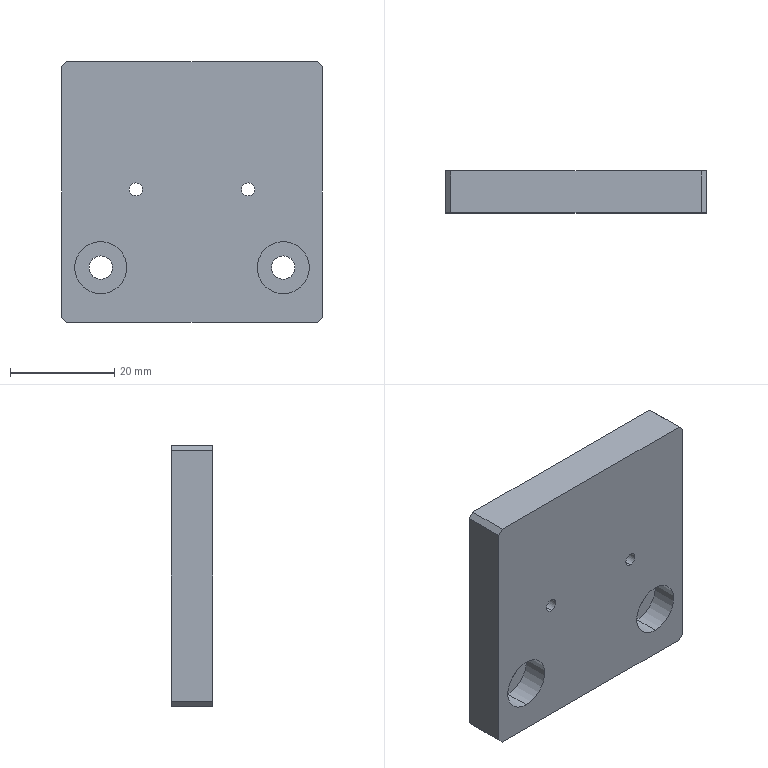Part | NX | features BREP 1 | 1 solid | 24 faces | box 50 x 8 x 50 mm | volume 19025 mm3 | plane 12 | cylinder 12 | commonest cylinder face diameters 2.5 x4 4.5 x4 10 x4
STEP:
#1=CARTESIAN_POINT('',(24.,8.,25.));
#2=VERTEX_POINT('',#1);
#3=CARTESIAN_POINT('',(25.,8.,24.));
#4=VERTEX_POINT('',#3);
#5=CARTESIAN_POINT('',(24.5,8.,24.5));
#6=DIRECTION('',(0.7071,0.,-0.7071));
#7=VECTOR('',#6,1000.);
#8=LINE('',#5,#7);
#9=EDGE_CURVE('',#2,#4,#8,.T.);
#10=ORIENTED_EDGE('',*,*,#9,.F.);
#11=CARTESIAN_POINT('',(24.,0.,25.));
#12=VERTEX_POINT('',#11);
#13=CARTESIAN_POINT('',(24.,8.,25.));
#14=DIRECTION('',(0.,1.,0.));
#15=VECTOR('',#14,1000.);
#16=LINE('',#13,#15);
#17=EDGE_CURVE('',#12,#2,#16,.T.);
#18=ORIENTED_EDGE('',*,*,#17,.F.);
#19=CARTESIAN_POINT('',(25.,0.,24.));
#20=VERTEX_POINT('',#19);
#21=CARTESIAN_POINT('',(25.,0.,24.));
#22=DIRECTION('',(-0.7071,0.,0.7071));
#23=VECTOR('',#22,1000.);
#24=LINE('',#21,#23);
#25=EDGE_CURVE('',#20,#12,#24,.T.);
#26=ORIENTED_EDGE('',*,*,#25,.F.);
#27=CARTESIAN_POINT('',(25.,8.,24.));
#28=DIRECTION('',(0.,-1.,0.));
#29=VECTOR('',#28,1000.);
#30=LINE('',#27,#29);
#31=EDGE_CURVE('',#4,#20,#30,.T.);
#32=ORIENTED_EDGE('',*,*,#31,.F.);
#33=EDGE_LOOP('',(#10,#18,#26,#32));
#34=FACE_BOUND('',#33,.T.);
#35=CARTESIAN_POINT('',(25.,8.,24.));
#36=DIRECTION('',(-0.7071,0.,-0.7071));
#37=DIRECTION('',(0.,-1.,0.));
#38=AXIS2_PLACEMENT_3D('',#35,#36,#37);
#39=PLANE('',#38);
#40=ADVANCED_FACE('',(#34),#39,.F.);
#41=CARTESIAN_POINT('',(-25.,8.,24.));
#42=VERTEX_POINT('',#41);
#43=CARTESIAN_POINT('',(-24.,8.,25.));
#44=VERTEX_POINT('',#43);
#45=CARTESIAN_POINT('',(-24.5,8.,24.5));
#46=DIRECTION('',(0.7071,0.,0.7071));
#47=VECTOR('',#46,1000.);
#48=LINE('',#45,#47);
#49=EDGE_CURVE('',#42,#44,#48,.T.);
#50=ORIENTED_EDGE('',*,*,#49,.F.);
#51=CARTESIAN_POINT('',(-25.,0.,24.));
#52=VERTEX_POINT('',#51);
#53=CARTESIAN_POINT('',(-25.,8.,24.));
#54=DIRECTION('',(0.,1.,0.));
#55=VECTOR('',#54,1000.);
#56=LINE('',#53,#55);
#57=EDGE_CURVE('',#52,#42,#56,.T.);
#58=ORIENTED_EDGE('',*,*,#57,.F.);
#59=CARTESIAN_POINT('',(-24.,0.,25.));
#60=VERTEX_POINT('',#59);
#61=CARTESIAN_POINT('',(-24.,0.,25.));
#62=DIRECTION('',(-0.7071,0.,-0.7071));
#63=VECTOR('',#62,1000.);
#64=LINE('',#61,#63);
#65=EDGE_CURVE('',#60,#52,#64,.T.);
#66=ORIENTED_EDGE('',*,*,#65,.F.);
#67=CARTESIAN_POINT('',(-24.,8.,25.));
#68=DIRECTION('',(0.,-1.,0.));
#69=VECTOR('',#68,1000.);
#70=LINE('',#67,#69);
#71=EDGE_CURVE('',#44,#60,#70,.T.);
#72=ORIENTED_EDGE('',*,*,#71,.F.);
#73=EDGE_LOOP('',(#50,#58,#66,#72));
#74=FACE_BOUND('',#73,.T.);
#75=CARTESIAN_POINT('',(-24.,8.,25.));
#76=DIRECTION('',(0.7071,0.,-0.7071));
#77=DIRECTION('',(0.,-1.,0.));
#78=AXIS2_PLACEMENT_3D('',#75,#76,#77);
#79=PLANE('',#78);
#80=ADVANCED_FACE('',(#74),#79,.F.);
#81=CARTESIAN_POINT('',(-24.,8.,-25.));
#82=VERTEX_POINT('',#81);
#83=CARTESIAN_POINT('',(-25.,8.,-24.));
#84=VERTEX_POINT('',#83);
#85=CARTESIAN_POINT('',(-24.5,8.,-24.5));
#86=DIRECTION('',(-0.7071,0.,0.7071));
#87=VECTOR('',#86,1000.);
#88=LINE('',#85,#87);
#89=EDGE_CURVE('',#82,#84,#88,.T.);
#90=ORIENTED_EDGE('',*,*,#89,.F.);
#91=CARTESIAN_POINT('',(-24.,0.,-25.));
#92=VERTEX_POINT('',#91);
#93=CARTESIAN_POINT('',(-24.,8.,-25.));
#94=DIRECTION('',(0.,1.,0.));
#95=VECTOR('',#94,1000.);
#96=LINE('',#93,#95);
#97=EDGE_CURVE('',#92,#82,#96,.T.);
#98=ORIENTED_EDGE('',*,*,#97,.F.);
#99=CARTESIAN_POINT('',(-25.,0.,-24.));
#100=VERTEX_POINT('',#99);
#101=CARTESIAN_POINT('',(-25.,0.,-24.));
#102=DIRECTION('',(0.7071,0.,-0.7071));
#103=VECTOR('',#102,1000.);
#104=LINE('',#101,#103);
#105=EDGE_CURVE('',#100,#92,#104,.T.);
#106=ORIENTED_EDGE('',*,*,#105,.F.);
#107=CARTESIAN_POINT('',(-25.,8.,-24.));
#108=DIRECTION('',(0.,-1.,0.));
#109=VECTOR('',#108,1000.);
#110=LINE('',#107,#109);
#111=EDGE_CURVE('',#84,#100,#110,.T.);
#112=ORIENTED_EDGE('',*,*,#111,.F.);
#113=EDGE_LOOP('',(#90,#98,#106,#112));
#114=FACE_BOUND('',#113,.T.);
#115=CARTESIAN_POINT('',(-25.,8.,-24.));
#116=DIRECTION('',(0.7071,0.,0.7071));
#117=DIRECTION('',(0.,-1.,0.));
#118=AXIS2_PLACEMENT_3D('',#115,#116,#117);
#119=PLANE('',#118);
#120=ADVANCED_FACE('',(#114),#119,.F.);
#121=CARTESIAN_POINT('',(25.,8.,-24.));
#122=VERTEX_POINT('',#121);
#123=CARTESIAN_POINT('',(24.,8.,-25.));
#124=VERTEX_POINT('',#123);
#125=CARTESIAN_POINT('',(24.5,8.,-24.5));
#126=DIRECTION('',(-0.7071,0.,-0.7071));
#127=VECTOR('',#126,1000.);
#128=LINE('',#125,#127);
#129=EDGE_CURVE('',#122,#124,#128,.T.);
#130=ORIENTED_EDGE('',*,*,#129,.F.);
#131=CARTESIAN_POINT('',(25.,0.,-24.));
#132=VERTEX_POINT('',#131);
#133=CARTESIAN_POINT('',(25.,8.,-24.));
#134=DIRECTION('',(0.,1.,0.));
#135=VECTOR('',#134,1000.);
#136=LINE('',#133,#135);
#137=EDGE_CURVE('',#132,#122,#136,.T.);
#138=ORIENTED_EDGE('',*,*,#137,.F.);
#139=CARTESIAN_POINT('',(24.,0.,-25.));
#140=VERTEX_POINT('',#139);
#141=CARTESIAN_POINT('',(24.,0.,-25.));
#142=DIRECTION('',(0.7071,0.,0.7071));
#143=VECTOR('',#142,1000.);
#144=LINE('',#141,#143);
#145=EDGE_CURVE('',#140,#132,#144,.T.);
#146=ORIENTED_EDGE('',*,*,#145,.F.);
#147=CARTESIAN_POINT('',(24.,8.,-25.));
#148=DIRECTION('',(0.,-1.,0.));
#149=VECTOR('',#148,1000.);
#150=LINE('',#147,#149);
#151=EDGE_CURVE('',#124,#140,#150,.T.);
#152=ORIENTED_EDGE('',*,*,#151,.F.);
#153=EDGE_LOOP('',(#130,#138,#146,#152));
#154=FACE_BOUND('',#153,.T.);
#155=CARTESIAN_POINT('',(24.,8.,-25.));
#156=DIRECTION('',(-0.7071,0.,0.7071));
#157=DIRECTION('',(0.,-1.,0.));
#158=AXIS2_PLACEMENT_3D('',#155,#156,#157);
#159=PLANE('',#158);
#160=ADVANCED_FACE('',(#154),#159,.F.);
#161=CARTESIAN_POINT('',(10.75,8.,1.75));
#162=VERTEX_POINT('',#161);
#163=CARTESIAN_POINT('',(10.75,0.,1.75));
#164=VERTEX_POINT('',#163);
#165=CARTESIAN_POINT('',(10.75,0.,1.75));
#166=DIRECTION('',(0.,-1.,0.));
#167=VECTOR('',#166,1000.);
#168=LINE('',#165,#167);
#169=EDGE_CURVE('',#162,#164,#168,.T.);
#170=ORIENTED_EDGE('',*,*,#169,.F.);
#171=CARTESIAN_POINT('',(10.75,8.,-0.75));
#172=VERTEX_POINT('',#171);
#173=CARTESIAN_POINT('',(10.75,8.,0.5));
#174=DIRECTION('',(0.,-1.,0.));
#175=DIRECTION('',(0.,0.,-1.));
#176=AXIS2_PLACEMENT_3D('',#173,#174,#175);
#177=CIRCLE('',#176,1.25);
#178=EDGE_CURVE('',#172,#162,#177,.T.);
#179=ORIENTED_EDGE('',*,*,#178,.F.);
#180=CARTESIAN_POINT('',(10.75,0.,-0.75));
#181=VERTEX_POINT('',#180);
#182=CARTESIAN_POINT('',(10.75,0.,-0.75));
#183=DIRECTION('',(0.,-1.,0.));
#184=VECTOR('',#183,1000.);
#185=LINE('',#182,#184);
#186=EDGE_CURVE('',#172,#181,#185,.T.);
#187=ORIENTED_EDGE('',*,*,#186,.T.);
#188=CARTESIAN_POINT('',(10.75,0.,0.5));
#189=DIRECTION('',(0.,-1.,0.));
#190=DIRECTION('',(0.,0.,-1.));
#191=AXIS2_PLACEMENT_3D('',#188,#189,#190);
#192=CIRCLE('',#191,1.25);
#193=EDGE_CURVE('',#181,#164,#192,.T.);
#194=ORIENTED_EDGE('',*,*,#193,.T.);
#195=EDGE_LOOP('',(#170,#179,#187,#194));
#196=FACE_BOUND('',#195,.T.);
#197=CARTESIAN_POINT('',(10.75,0.,0.5));
#198=DIRECTION('',(0.,-1.,0.));
#199=DIRECTION('',(0.,0.,-1.));
#200=AXIS2_PLACEMENT_3D('',#197,#198,#199);
#201=CYLINDRICAL_SURFACE('',#200,1.25);
#202=ADVANCED_FACE('',(#196),#201,.F.);
#203=CARTESIAN_POINT('',(-10.75,8.,1.75));
#204=VERTEX_POINT('',#203);
#205=CARTESIAN_POINT('',(-10.75,0.,1.75));
#206=VERTEX_POINT('',#205);
#207=CARTESIAN_POINT('',(-10.75,0.,1.75));
#208=DIRECTION('',(0.,-1.,0.));
#209=VECTOR('',#208,1000.);
#210=LINE('',#207,#209);
#211=EDGE_CURVE('',#204,#206,#210,.T.);
#212=ORIENTED_EDGE('',*,*,#211,.F.);
#213=CARTESIAN_POINT('',(-10.75,8.,-0.75));
#214=VERTEX_POINT('',#213);
#215=CARTESIAN_POINT('',(-10.75,8.,0.5));
#216=DIRECTION('',(0.,-1.,0.));
#217=DIRECTION('',(0.,0.,-1.));
#218=AXIS2_PLACEMENT_3D('',#215,#216,#217);
#219=CIRCLE('',#218,1.25);
#220=EDGE_CURVE('',#214,#204,#219,.T.);
#221=ORIENTED_EDGE('',*,*,#220,.F.);
#222=CARTESIAN_POINT('',(-10.75,0.,-0.75));
#223=VERTEX_POINT('',#222);
#224=CARTESIAN_POINT('',(-10.75,0.,-0.75));
#225=DIRECTION('',(0.,-1.,0.));
#226=VECTOR('',#225,1000.);
#227=LINE('',#224,#226);
#228=EDGE_CURVE('',#214,#223,#227,.T.);
#229=ORIENTED_EDGE('',*,*,#228,.T.);
#230=CARTESIAN_POINT('',(-10.75,0.,0.5));
#231=DIRECTION('',(0.,-1.,0.));
#232=DIRECTION('',(0.,0.,-1.));
#233=AXIS2_PLACEMENT_3D('',#230,#231,#232);
#234=CIRCLE('',#233,1.25);
#235=EDGE_CURVE('',#223,#206,#234,.T.);
#236=ORIENTED_EDGE('',*,*,#235,.T.);
#237=EDGE_LOOP('',(#212,#221,#229,#236));
#238=FACE_BOUND('',#237,.T.);
#239=CARTESIAN_POINT('',(-10.75,0.,0.5));
#240=DIRECTION('',(0.,-1.,0.));
#241=DIRECTION('',(0.,0.,-1.));
#242=AXIS2_PLACEMENT_3D('',#239,#240,#241);
#243=CYLINDRICAL_SURFACE('',#242,1.25);
#244=ADVANCED_FACE('',(#238),#243,.F.);
#245=CARTESIAN_POINT('',(17.5,5.,-9.5));
#246=VERTEX_POINT('',#245);
#247=CARTESIAN_POINT('',(17.5,0.,-9.5));
#248=VERTEX_POINT('',#247);
#249=CARTESIAN_POINT('',(17.5,0.,-9.5));
#250=DIRECTION('',(0.,-1.,0.));
#251=VECTOR('',#250,1000.);
#252=LINE('',#249,#251);
#253=EDGE_CURVE('',#246,#248,#252,.T.);
#254=ORIENTED_EDGE('',*,*,#253,.F.);
#255=CARTESIAN_POINT('',(17.5,5.,-19.5));
#256=VERTEX_POINT('',#255);
#257=CARTESIAN_POINT('',(17.5,5.,-14.5));
#258=DIRECTION('',(0.,-1.,0.));
#259=DIRECTION('',(0.,0.,-1.));
#260=AXIS2_PLACEMENT_3D('',#257,#258,#259);
#261=CIRCLE('',#260,5.);
#262=EDGE_CURVE('',#256,#246,#261,.T.);
#263=ORIENTED_EDGE('',*,*,#262,.F.);
#264=CARTESIAN_POINT('',(17.5,0.,-19.5));
#265=VERTEX_POINT('',#264);
#266=CARTESIAN_POINT('',(17.5,0.,-19.5));
#267=DIRECTION('',(0.,-1.,0.));
#268=VECTOR('',#267,1000.);
#269=LINE('',#266,#268);
#270=EDGE_CURVE('',#256,#265,#269,.T.);
#271=ORIENTED_EDGE('',*,*,#270,.T.);
#272=CARTESIAN_POINT('',(17.5,0.,-14.5));
#273=DIRECTION('',(0.,-1.,0.));
#274=DIRECTION('',(0.,0.,-1.));
#275=AXIS2_PLACEMENT_3D('',#272,#273,#274);
#276=CIRCLE('',#275,5.);
#277=EDGE_CURVE('',#265,#248,#276,.T.);
#278=ORIENTED_EDGE('',*,*,#277,.T.);
#279=EDGE_LOOP('',(#254,#263,#271,#278));
#280=FACE_BOUND('',#279,.T.);
#281=CARTESIAN_POINT('',(17.5,0.,-14.5));
#282=DIRECTION('',(0.,-1.,0.));
#283=DIRECTION('',(0.,0.,-1.));
#284=AXIS2_PLACEMENT_3D('',#281,#282,#283);
#285=CYLINDRICAL_SURFACE('',#284,5.);
#286=ADVANCED_FACE('',(#280),#285,.F.);
#287=ORIENTED_EDGE('',*,*,#262,.T.);
#288=CARTESIAN_POINT('',(17.5,5.,-14.5));
#289=DIRECTION('',(0.,-1.,0.));
#290=DIRECTION('',(0.,0.,-1.));
#291=AXIS2_PLACEMENT_3D('',#288,#289,#290);
#292=CIRCLE('',#291,5.);
#293=EDGE_CURVE('',#246,#256,#292,.T.);
#294=ORIENTED_EDGE('',*,*,#293,.T.);
#295=EDGE_LOOP('',(#287,#294));
#296=FACE_BOUND('',#295,.T.);
#297=CARTESIAN_POINT('',(17.5,5.,-16.75));
#298=VERTEX_POINT('',#297);
#299=CARTESIAN_POINT('',(17.5,5.,-12.25));
#300=VERTEX_POINT('',#299);
#301=CARTESIAN_POINT('',(17.5,5.,-14.5));
#302=DIRECTION('',(0.,-1.,0.));
#303=DIRECTION('',(0.,0.,-1.));
#304=AXIS2_PLACEMENT_3D('',#301,#302,#303);
#305=CIRCLE('',#304,2.25);
#306=EDGE_CURVE('',#298,#300,#305,.T.);
#307=ORIENTED_EDGE('',*,*,#306,.F.);
#308=CARTESIAN_POINT('',(17.5,5.,-14.5));
#309=DIRECTION('',(0.,-1.,0.));
#310=DIRECTION('',(0.,0.,-1.));
#311=AXIS2_PLACEMENT_3D('',#308,#309,#310);
#312=CIRCLE('',#311,2.25);
#313=EDGE_CURVE('',#300,#298,#312,.T.);
#314=ORIENTED_EDGE('',*,*,#313,.F.);
#315=EDGE_LOOP('',(#307,#314));
#316=FACE_BOUND('',#315,.T.);
#317=CARTESIAN_POINT('',(19.75,5.,-14.5));
#318=DIRECTION('',(0.,1.,0.));
#319=DIRECTION('',(0.,0.,1.));
#320=AXIS2_PLACEMENT_3D('',#317,#318,#319);
#321=PLANE('',#320);
#322=ADVANCED_FACE('',(#296,#316),#321,.F.);
#323=CARTESIAN_POINT('',(17.5,8.,-12.25));
#324=VERTEX_POINT('',#323);
#325=CARTESIAN_POINT('',(17.5,0.,-12.25));
#326=DIRECTION('',(0.,-1.,0.));
#327=VECTOR('',#326,1000.);
#328=LINE('',#325,#327);
#329=EDGE_CURVE('',#324,#300,#328,.T.);
#330=ORIENTED_EDGE('',*,*,#329,.F.);
#331=CARTESIAN_POINT('',(17.5,8.,-16.75));
#332=VERTEX_POINT('',#331);
#333=CARTESIAN_POINT('',(17.5,8.,-14.5));
#334=DIRECTION('',(0.,-1.,0.));
#335=DIRECTION('',(0.,0.,-1.));
#336=AXIS2_PLACEMENT_3D('',#333,#334,#335);
#337=CIRCLE('',#336,2.25);
#338=EDGE_CURVE('',#332,#324,#337,.T.);
#339=ORIENTED_EDGE('',*,*,#338,.F.);
#340=CARTESIAN_POINT('',(17.5,0.,-16.75));
#341=DIRECTION('',(0.,-1.,0.));
#342=VECTOR('',#341,1000.);
#343=LINE('',#340,#342);
#344=EDGE_CURVE('',#332,#298,#343,.T.);
#345=ORIENTED_EDGE('',*,*,#344,.T.);
#346=ORIENTED_EDGE('',*,*,#306,.T.);
#347=EDGE_LOOP('',(#330,#339,#345,#346));
#348=FACE_BOUND('',#347,.T.);
#349=CARTESIAN_POINT('',(17.5,0.,-14.5));
#350=DIRECTION('',(0.,-1.,0.));
#351=DIRECTION('',(0.,0.,-1.));
#352=AXIS2_PLACEMENT_3D('',#349,#350,#351);
#353=CYLINDRICAL_SURFACE('',#352,2.25);
#354=ADVANCED_FACE('',(#348),#353,.F.);
#355=CARTESIAN_POINT('',(-17.5,5.,-9.5));
#356=VERTEX_POINT('',#355);
#357=CARTESIAN_POINT('',(-17.5,0.,-9.5));
#358=VERTEX_POINT('',#357);
#359=CARTESIAN_POINT('',(-17.5,0.,-9.5));
#360=DIRECTION('',(0.,-1.,0.));
#361=VECTOR('',#360,1000.);
#362=LINE('',#359,#361);
#363=EDGE_CURVE('',#356,#358,#362,.T.);
#364=ORIENTED_EDGE('',*,*,#363,.F.);
#365=CARTESIAN_POINT('',(-17.5,5.,-19.5));
#366=VERTEX_POINT('',#365);
#367=CARTESIAN_POINT('',(-17.5,5.,-14.5));
#368=DIRECTION('',(0.,-1.,0.));
#369=DIRECTION('',(0.,0.,-1.));
#370=AXIS2_PLACEMENT_3D('',#367,#368,#369);
#371=CIRCLE('',#370,5.);
#372=EDGE_CURVE('',#366,#356,#371,.T.);
#373=ORIENTED_EDGE('',*,*,#372,.F.);
#374=CARTESIAN_POINT('',(-17.5,0.,-19.5));
#375=VERTEX_POINT('',#374);
#376=CARTESIAN_POINT('',(-17.5,0.,-19.5));
#377=DIRECTION('',(0.,-1.,0.));
#378=VECTOR('',#377,1000.);
#379=LINE('',#376,#378);
#380=EDGE_CURVE('',#366,#375,#379,.T.);
#381=ORIENTED_EDGE('',*,*,#380,.T.);
#382=CARTESIAN_POINT('',(-17.5,0.,-14.5));
#383=DIRECTION('',(0.,-1.,0.));
#384=DIRECTION('',(0.,0.,-1.));
#385=AXIS2_PLACEMENT_3D('',#382,#383,#384);
#386=CIRCLE('',#385,5.);
#387=EDGE_CURVE('',#375,#358,#386,.T.);
#388=ORIENTED_EDGE('',*,*,#387,.T.);
#389=EDGE_LOOP('',(#364,#373,#381,#388));
#390=FACE_BOUND('',#389,.T.);
#391=CARTESIAN_POINT('',(-17.5,0.,-14.5));
#392=DIRECTION('',(0.,-1.,0.));
#393=DIRECTION('',(0.,0.,-1.));
#394=AXIS2_PLACEMENT_3D('',#391,#392,#393);
#395=CYLINDRICAL_SURFACE('',#394,5.);
#396=ADVANCED_FACE('',(#390),#395,.F.);
#397=ORIENTED_EDGE('',*,*,#372,.T.);
#398=CARTESIAN_POINT('',(-17.5,5.,-14.5));
#399=DIRECTION('',(0.,-1.,0.));
#400=DIRECTION('',(0.,0.,-1.));
#401=AXIS2_PLACEMENT_3D('',#398,#399,#400);
#402=CIRCLE('',#401,5.);
#403=EDGE_CURVE('',#356,#366,#402,.T.);
#404=ORIENTED_EDGE('',*,*,#403,.T.);
#405=EDGE_LOOP('',(#397,#404));
#406=FACE_BOUND('',#405,.T.);
#407=CARTESIAN_POINT('',(-17.5,5.,-16.75));
#408=VERTEX_POINT('',#407);
#409=CARTESIAN_POINT('',(-17.5,5.,-12.25));
#410=VERTEX_POINT('',#409);
#411=CARTESIAN_POINT('',(-17.5,5.,-14.5));
#412=DIRECTION('',(0.,-1.,0.));
#413=DIRECTION('',(0.,0.,-1.));
#414=AXIS2_PLACEMENT_3D('',#411,#412,#413);
#415=CIRCLE('',#414,2.25);
#416=EDGE_CURVE('',#408,#410,#415,.T.);
#417=ORIENTED_EDGE('',*,*,#416,.F.);
#418=CARTESIAN_POINT('',(-17.5,5.,-14.5));
#419=DIRECTION('',(0.,-1.,0.));
#420=DIRECTION('',(0.,0.,-1.));
#421=AXIS2_PLACEMENT_3D('',#418,#419,#420);
#422=CIRCLE('',#421,2.25);
#423=EDGE_CURVE('',#410,#408,#422,.T.);
#424=ORIENTED_EDGE('',*,*,#423,.F.);
#425=EDGE_LOOP('',(#417,#424));
#426=FACE_BOUND('',#425,.T.);
#427=CARTESIAN_POINT('',(-15.25,5.,-14.5));
#428=DIRECTION('',(0.,1.,0.));
#429=DIRECTION('',(0.,0.,1.));
#430=AXIS2_PLACEMENT_3D('',#427,#428,#429);
#431=PLANE('',#430);
#432=ADVANCED_FACE('',(#406,#426),#431,.F.);
#433=CARTESIAN_POINT('',(-17.5,8.,-12.25));
#434=VERTEX_POINT('',#433);
#435=CARTESIAN_POINT('',(-17.5,0.,-12.25));
#436=DIRECTION('',(0.,-1.,0.));
#437=VECTOR('',#436,1000.);
#438=LINE('',#435,#437);
#439=EDGE_CURVE('',#434,#410,#438,.T.);
#440=ORIENTED_EDGE('',*,*,#439,.F.);
#441=CARTESIAN_POINT('',(-17.5,8.,-16.75));
#442=VERTEX_POINT('',#441);
#443=CARTESIAN_POINT('',(-17.5,8.,-14.5));
#444=DIRECTION('',(0.,-1.,0.));
#445=DIRECTION('',(0.,0.,-1.));
#446=AXIS2_PLACEMENT_3D('',#443,#444,#445);
#447=CIRCLE('',#446,2.25);
#448=EDGE_CURVE('',#442,#434,#447,.T.);
#449=ORIENTED_EDGE('',*,*,#448,.F.);
#450=CARTESIAN_POINT('',(-17.5,0.,-16.75));
#451=DIRECTION('',(0.,-1.,0.));
#452=VECTOR('',#451,1000.);
#453=LINE('',#450,#452);
#454=EDGE_CURVE('',#442,#408,#453,.T.);
#455=ORIENTED_EDGE('',*,*,#454,.T.);
#456=ORIENTED_EDGE('',*,*,#416,.T.);
#457=EDGE_LOOP('',(#440,#449,#455,#456));
#458=FACE_BOUND('',#457,.T.);
#459=CARTESIAN_POINT('',(-17.5,0.,-14.5));
#460=DIRECTION('',(0.,-1.,0.));
#461=DIRECTION('',(0.,0.,-1.));
#462=AXIS2_PLACEMENT_3D('',#459,#460,#461);
#463=CYLINDRICAL_SURFACE('',#462,2.25);
#464=ADVANCED_FACE('',(#458),#463,.F.);
#465=CARTESIAN_POINT('',(25.,0.,-25.));
#466=DIRECTION('',(-1.,0.,0.));
#467=VECTOR('',#466,1000.);
#468=LINE('',#465,#467);
#469=EDGE_CURVE('',#140,#92,#468,.T.);
#470=ORIENTED_EDGE('',*,*,#469,.F.);
#471=ORIENTED_EDGE('',*,*,#145,.T.);
#472=CARTESIAN_POINT('',(25.,0.,25.));
#473=DIRECTION('',(0.,0.,-1.));
#474=VECTOR('',#473,1000.);
#475=LINE('',#472,#474);
#476=EDGE_CURVE('',#20,#132,#475,.T.);
#477=ORIENTED_EDGE('',*,*,#476,.F.);
#478=ORIENTED_EDGE('',*,*,#25,.T.);
#479=CARTESIAN_POINT('',(25.,0.,25.));
#480=DIRECTION('',(1.,0.,0.));
#481=VECTOR('',#480,1000.);
#482=LINE('',#479,#481);
#483=EDGE_CURVE('',#60,#12,#482,.T.);
#484=ORIENTED_EDGE('',*,*,#483,.F.);
#485=ORIENTED_EDGE('',*,*,#65,.T.);
#486=CARTESIAN_POINT('',(-25.,0.,25.));
#487=DIRECTION('',(0.,0.,1.));
#488=VECTOR('',#487,1000.);
#489=LINE('',#486,#488);
#490=EDGE_CURVE('',#100,#52,#489,.T.);
#491=ORIENTED_EDGE('',*,*,#490,.F.);
#492=ORIENTED_EDGE('',*,*,#105,.T.);
#493=EDGE_LOOP('',(#470,#471,#477,#478,#484,#485,#491,#492));
#494=FACE_BOUND('',#493,.T.);
#495=ORIENTED_EDGE('',*,*,#387,.F.);
#496=CARTESIAN_POINT('',(-17.5,0.,-14.5));
#497=DIRECTION('',(0.,-1.,0.));
#498=DIRECTION('',(0.,0.,-1.));
#499=AXIS2_PLACEMENT_3D('',#496,#497,#498);
#500=CIRCLE('',#499,5.);
#501=EDGE_CURVE('',#358,#375,#500,.T.);
#502=ORIENTED_EDGE('',*,*,#501,.F.);
#503=EDGE_LOOP('',(#495,#502));
#504=FACE_BOUND('',#503,.T.);
#505=ORIENTED_EDGE('',*,*,#277,.F.);
#506=CARTESIAN_POINT('',(17.5,0.,-14.5));
#507=DIRECTION('',(0.,-1.,0.));
#508=DIRECTION('',(0.,0.,-1.));
#509=AXIS2_PLACEMENT_3D('',#506,#507,#508);
#510=CIRCLE('',#509,5.);
#511=EDGE_CURVE('',#248,#265,#510,.T.);
#512=ORIENTED_EDGE('',*,*,#511,.F.);
#513=EDGE_LOOP('',(#505,#512));
#514=FACE_BOUND('',#513,.T.);
#515=ORIENTED_EDGE('',*,*,#235,.F.);
#516=CARTESIAN_POINT('',(-10.75,0.,0.5));
#517=DIRECTION('',(0.,-1.,0.));
#518=DIRECTION('',(0.,0.,-1.));
#519=AXIS2_PLACEMENT_3D('',#516,#517,#518);
#520=CIRCLE('',#519,1.25);
#521=EDGE_CURVE('',#206,#223,#520,.T.);
#522=ORIENTED_EDGE('',*,*,#521,.F.);
#523=EDGE_LOOP('',(#515,#522));
#524=FACE_BOUND('',#523,.T.);
#525=ORIENTED_EDGE('',*,*,#193,.F.);
#526=CARTESIAN_POINT('',(10.75,0.,0.5));
#527=DIRECTION('',(0.,-1.,0.));
#528=DIRECTION('',(0.,0.,-1.));
#529=AXIS2_PLACEMENT_3D('',#526,#527,#528);
#530=CIRCLE('',#529,1.25);
#531=EDGE_CURVE('',#164,#181,#530,.T.);
#532=ORIENTED_EDGE('',*,*,#531,.F.);
#533=EDGE_LOOP('',(#525,#532));
#534=FACE_BOUND('',#533,.T.);
#535=CARTESIAN_POINT('',(0.,0.,0.));
#536=DIRECTION('',(0.,1.,0.));
#537=DIRECTION('',(0.,0.,1.));
#538=AXIS2_PLACEMENT_3D('',#535,#536,#537);
#539=PLANE('',#538);
#540=ADVANCED_FACE('',(#494,#504,#514,#524,#534),#539,.F.);
#541=CARTESIAN_POINT('',(25.,8.,25.));
#542=DIRECTION('',(0.,0.,-1.));
#543=VECTOR('',#542,1000.);
#544=LINE('',#541,#543);
#545=EDGE_CURVE('',#4,#122,#544,.T.);
#546=ORIENTED_EDGE('',*,*,#545,.T.);
#547=ORIENTED_EDGE('',*,*,#129,.T.);
#548=CARTESIAN_POINT('',(25.,8.,-25.));
#549=DIRECTION('',(-1.,0.,0.));
#550=VECTOR('',#549,1000.);
#551=LINE('',#548,#550);
#552=EDGE_CURVE('',#124,#82,#551,.T.);
#553=ORIENTED_EDGE('',*,*,#552,.T.);
#554=ORIENTED_EDGE('',*,*,#89,.T.);
#555=CARTESIAN_POINT('',(-25.,8.,25.));
#556=DIRECTION('',(0.,0.,1.));
#557=VECTOR('',#556,1000.);
#558=LINE('',#555,#557);
#559=EDGE_CURVE('',#84,#42,#558,.T.);
#560=ORIENTED_EDGE('',*,*,#559,.T.);
#561=ORIENTED_EDGE('',*,*,#49,.T.);
#562=CARTESIAN_POINT('',(25.,8.,25.));
#563=DIRECTION('',(1.,0.,0.));
#564=VECTOR('',#563,1000.);
#565=LINE('',#562,#564);
#566=EDGE_CURVE('',#44,#2,#565,.T.);
#567=ORIENTED_EDGE('',*,*,#566,.T.);
#568=ORIENTED_EDGE('',*,*,#9,.T.);
#569=EDGE_LOOP('',(#546,#547,#553,#554,#560,#561,#567,#568));
#570=FACE_BOUND('',#569,.T.);
#571=ORIENTED_EDGE('',*,*,#448,.T.);
#572=CARTESIAN_POINT('',(-17.5,8.,-14.5));
#573=DIRECTION('',(0.,-1.,0.));
#574=DIRECTION('',(0.,0.,-1.));
#575=AXIS2_PLACEMENT_3D('',#572,#573,#574);
#576=CIRCLE('',#575,2.25);
#577=EDGE_CURVE('',#434,#442,#576,.T.);
#578=ORIENTED_EDGE('',*,*,#577,.T.);
#579=EDGE_LOOP('',(#571,#578));
#580=FACE_BOUND('',#579,.T.);
#581=ORIENTED_EDGE('',*,*,#338,.T.);
#582=CARTESIAN_POINT('',(17.5,8.,-14.5));
#583=DIRECTION('',(0.,-1.,0.));
#584=DIRECTION('',(0.,0.,-1.));
#585=AXIS2_PLACEMENT_3D('',#582,#583,#584);
#586=CIRCLE('',#585,2.25);
#587=EDGE_CURVE('',#324,#332,#586,.T.);
#588=ORIENTED_EDGE('',*,*,#587,.T.);
#589=EDGE_LOOP('',(#581,#588));
#590=FACE_BOUND('',#589,.T.);
#591=ORIENTED_EDGE('',*,*,#220,.T.);
#592=CARTESIAN_POINT('',(-10.75,8.,0.5));
#593=DIRECTION('',(0.,-1.,0.));
#594=DIRECTION('',(0.,0.,-1.));
#595=AXIS2_PLACEMENT_3D('',#592,#593,#594);
#596=CIRCLE('',#595,1.25);
#597=EDGE_CURVE('',#204,#214,#596,.T.);
#598=ORIENTED_EDGE('',*,*,#597,.T.);
#599=EDGE_LOOP('',(#591,#598));
#600=FACE_BOUND('',#599,.T.);
#601=ORIENTED_EDGE('',*,*,#178,.T.);
#602=CARTESIAN_POINT('',(10.75,8.,0.5));
#603=DIRECTION('',(0.,-1.,0.));
#604=DIRECTION('',(0.,0.,-1.));
#605=AXIS2_PLACEMENT_3D('',#602,#603,#604);
#606=CIRCLE('',#605,1.25);
#607=EDGE_CURVE('',#162,#172,#606,.T.);
#608=ORIENTED_EDGE('',*,*,#607,.T.);
#609=EDGE_LOOP('',(#601,#608));
#610=FACE_BOUND('',#609,.T.);
#611=CARTESIAN_POINT('',(0.,8.,0.));
#612=DIRECTION('',(0.,1.,0.));
#613=DIRECTION('',(0.,0.,1.));
#614=AXIS2_PLACEMENT_3D('',#611,#612,#613);
#615=PLANE('',#614);
#616=ADVANCED_FACE('',(#570,#580,#590,#600,#610),#615,.T.);
#617=ORIENTED_EDGE('',*,*,#552,.F.);
#618=ORIENTED_EDGE('',*,*,#151,.T.);
#619=ORIENTED_EDGE('',*,*,#469,.T.);
#620=ORIENTED_EDGE('',*,*,#97,.T.);
#621=EDGE_LOOP('',(#617,#618,#619,#620));
#622=FACE_BOUND('',#621,.T.);
#623=CARTESIAN_POINT('',(25.,8.,-25.));
#624=DIRECTION('',(0.,0.,1.));
#625=DIRECTION('',(1.,0.,0.));
#626=AXIS2_PLACEMENT_3D('',#623,#624,#625);
#627=PLANE('',#626);
#628=ADVANCED_FACE('',(#622),#627,.F.);
#629=ORIENTED_EDGE('',*,*,#476,.T.);
#630=ORIENTED_EDGE('',*,*,#137,.T.);
#631=ORIENTED_EDGE('',*,*,#545,.F.);
#632=ORIENTED_EDGE('',*,*,#31,.T.);
#633=EDGE_LOOP('',(#629,#630,#631,#632));
#634=FACE_BOUND('',#633,.T.);
#635=CARTESIAN_POINT('',(25.,8.,25.));
#636=DIRECTION('',(-1.,0.,0.));
#637=DIRECTION('',(0.,0.,1.));
#638=AXIS2_PLACEMENT_3D('',#635,#636,#637);
#639=PLANE('',#638);
#640=ADVANCED_FACE('',(#634),#639,.F.);
#641=ORIENTED_EDGE('',*,*,#566,.F.);
#642=ORIENTED_EDGE('',*,*,#71,.T.);
#643=ORIENTED_EDGE('',*,*,#483,.T.);
#644=ORIENTED_EDGE('',*,*,#17,.T.);
#645=EDGE_LOOP('',(#641,#642,#643,#644));
#646=FACE_BOUND('',#645,.T.);
#647=CARTESIAN_POINT('',(25.,8.,25.));
#648=DIRECTION('',(0.,0.,-1.));
#649=DIRECTION('',(-1.,0.,0.));
#650=AXIS2_PLACEMENT_3D('',#647,#648,#649);
#651=PLANE('',#650);
#652=ADVANCED_FACE('',(#646),#651,.F.);
#653=ORIENTED_EDGE('',*,*,#559,.F.);
#654=ORIENTED_EDGE('',*,*,#111,.T.);
#655=ORIENTED_EDGE('',*,*,#490,.T.);
#656=ORIENTED_EDGE('',*,*,#57,.T.);
#657=EDGE_LOOP('',(#653,#654,#655,#656));
#658=FACE_BOUND('',#657,.T.);
#659=CARTESIAN_POINT('',(-25.,8.,25.));
#660=DIRECTION('',(1.,0.,0.));
#661=DIRECTION('',(0.,0.,-1.));
#662=AXIS2_PLACEMENT_3D('',#659,#660,#661);
#663=PLANE('',#662);
#664=ADVANCED_FACE('',(#658),#663,.F.);
#665=ORIENTED_EDGE('',*,*,#577,.F.);
#666=ORIENTED_EDGE('',*,*,#439,.T.);
#667=ORIENTED_EDGE('',*,*,#423,.T.);
#668=ORIENTED_EDGE('',*,*,#454,.F.);
#669=EDGE_LOOP('',(#665,#666,#667,#668));
#670=FACE_BOUND('',#669,.T.);
#671=CARTESIAN_POINT('',(-17.5,0.,-14.5));
#672=DIRECTION('',(0.,-1.,0.));
#673=DIRECTION('',(0.,0.,-1.));
#674=AXIS2_PLACEMENT_3D('',#671,#672,#673);
#675=CYLINDRICAL_SURFACE('',#674,2.25);
#676=ADVANCED_FACE('',(#670),#675,.F.);
#677=ORIENTED_EDGE('',*,*,#403,.F.);
#678=ORIENTED_EDGE('',*,*,#363,.T.);
#679=ORIENTED_EDGE('',*,*,#501,.T.);
#680=ORIENTED_EDGE('',*,*,#380,.F.);
#681=EDGE_LOOP('',(#677,#678,#679,#680));
#682=FACE_BOUND('',#681,.T.);
#683=CARTESIAN_POINT('',(-17.5,0.,-14.5));
#684=DIRECTION('',(0.,-1.,0.));
#685=DIRECTION('',(0.,0.,-1.));
#686=AXIS2_PLACEMENT_3D('',#683,#684,#685);
#687=CYLINDRICAL_SURFACE('',#686,5.);
#688=ADVANCED_FACE('',(#682),#687,.F.);
#689=ORIENTED_EDGE('',*,*,#587,.F.);
#690=ORIENTED_EDGE('',*,*,#329,.T.);
#691=ORIENTED_EDGE('',*,*,#313,.T.);
#692=ORIENTED_EDGE('',*,*,#344,.F.);
#693=EDGE_LOOP('',(#689,#690,#691,#692));
#694=FACE_BOUND('',#693,.T.);
#695=CARTESIAN_POINT('',(17.5,0.,-14.5));
#696=DIRECTION('',(0.,-1.,0.));
#697=DIRECTION('',(0.,0.,-1.));
#698=AXIS2_PLACEMENT_3D('',#695,#696,#697);
#699=CYLINDRICAL_SURFACE('',#698,2.25);
#700=ADVANCED_FACE('',(#694),#699,.F.);
#701=ORIENTED_EDGE('',*,*,#293,.F.);
#702=ORIENTED_EDGE('',*,*,#253,.T.);
#703=ORIENTED_EDGE('',*,*,#511,.T.);
#704=ORIENTED_EDGE('',*,*,#270,.F.);
#705=EDGE_LOOP('',(#701,#702,#703,#704));
#706=FACE_BOUND('',#705,.T.);
#707=CARTESIAN_POINT('',(17.5,0.,-14.5));
#708=DIRECTION('',(0.,-1.,0.));
#709=DIRECTION('',(0.,0.,-1.));
#710=AXIS2_PLACEMENT_3D('',#707,#708,#709);
#711=CYLINDRICAL_SURFACE('',#710,5.);
#712=ADVANCED_FACE('',(#706),#711,.F.);
#713=ORIENTED_EDGE('',*,*,#597,.F.);
#714=ORIENTED_EDGE('',*,*,#211,.T.);
#715=ORIENTED_EDGE('',*,*,#521,.T.);
#716=ORIENTED_EDGE('',*,*,#228,.F.);
#717=EDGE_LOOP('',(#713,#714,#715,#716));
#718=FACE_BOUND('',#717,.T.);
#719=CARTESIAN_POINT('',(-10.75,0.,0.5));
#720=DIRECTION('',(0.,-1.,0.));
#721=DIRECTION('',(0.,0.,-1.));
#722=AXIS2_PLACEMENT_3D('',#719,#720,#721);
#723=CYLINDRICAL_SURFACE('',#722,1.25);
#724=ADVANCED_FACE('',(#718),#723,.F.);
#725=ORIENTED_EDGE('',*,*,#607,.F.);
#726=ORIENTED_EDGE('',*,*,#169,.T.);
#727=ORIENTED_EDGE('',*,*,#531,.T.);
#728=ORIENTED_EDGE('',*,*,#186,.F.);
#729=EDGE_LOOP('',(#725,#726,#727,#728));
#730=FACE_BOUND('',#729,.T.);
#731=CARTESIAN_POINT('',(10.75,0.,0.5));
#732=DIRECTION('',(0.,-1.,0.));
#733=DIRECTION('',(0.,0.,-1.));
#734=AXIS2_PLACEMENT_3D('',#731,#732,#733);
#735=CYLINDRICAL_SURFACE('',#734,1.25);
#736=ADVANCED_FACE('',(#730),#735,.F.);
#737=CLOSED_SHELL('',(#40,#80,#120,#160,#202,#244,#286,#322,#354,#396,#432,#464,#540,#616,#628,#640,#652,#664,#676,#688,#700,#712,#724,#736));
#738=MANIFOLD_SOLID_BREP('',#737);
#739=(LENGTH_UNIT()NAMED_UNIT(*)SI_UNIT(.MILLI.,.METRE.));
#740=UNCERTAINTY_MEASURE_WITH_UNIT(LENGTH_MEASURE(0.00001),#739,'','');
#741=(NAMED_UNIT(*)PLANE_ANGLE_UNIT()SI_UNIT($,.RADIAN.));
#742=(NAMED_UNIT(*)SI_UNIT($,.STERADIAN.)SOLID_ANGLE_UNIT());
#743=(GEOMETRIC_REPRESENTATION_CONTEXT(3)GLOBAL_UNCERTAINTY_ASSIGNED_CONTEXT((#740))GLOBAL_UNIT_ASSIGNED_CONTEXT((#739,#741,#742))REPRESENTATION_CONTEXT('',''));
#744=ADVANCED_BREP_SHAPE_REPRESENTATION('',(#738),#743);